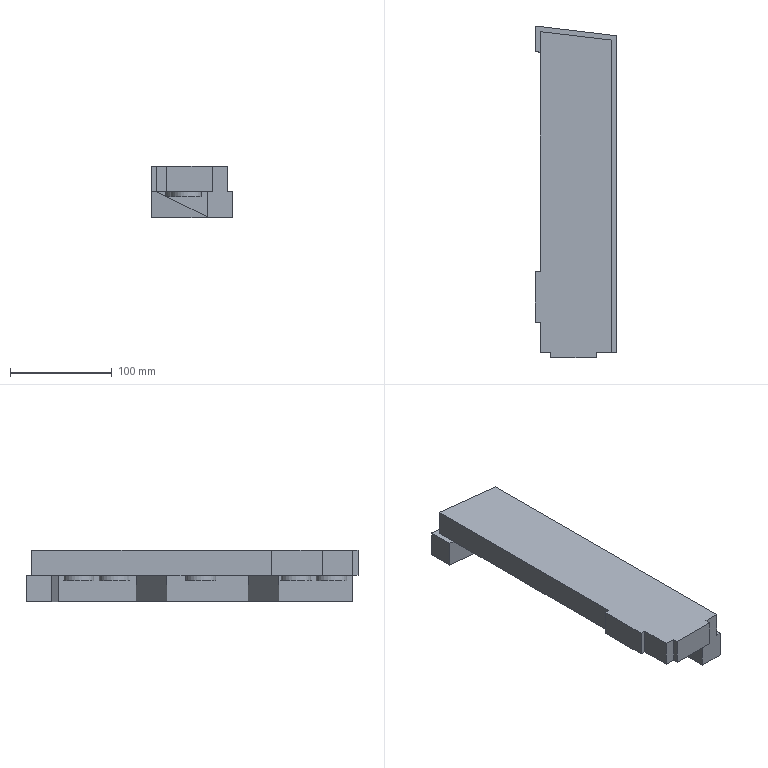Part | NX | features solid 2 | 1 solid | 39 faces | box 80 x 326.236 x 51 mm | volume 852017 mm3 | plane 31 | cylinder 5 | spline 3 | commonest cylinder face diameters 30 x5
STEP:
#1=CARTESIAN_POINT('',(-400.,-457.246,20.));
#2=VERTEX_POINT('',#1);
#3=CARTESIAN_POINT('',(-400.,-480.,20.));
#4=VERTEX_POINT('',#3);
#5=CARTESIAN_POINT('',(-400.,-457.246,20.));
#6=DIRECTION('',(0.,-1.,0.));
#7=VECTOR('',#6,1000.);
#8=LINE('',#5,#7);
#9=EDGE_CURVE('',#2,#4,#8,.T.);
#10=ORIENTED_EDGE('',*,*,#9,.T.);
#11=CARTESIAN_POINT('',(-400.,-480.,45.));
#12=VERTEX_POINT('',#11);
#13=CARTESIAN_POINT('',(-400.,-480.,20.));
#14=DIRECTION('',(0.,0.,-1.));
#15=VECTOR('',#14,1000.);
#16=LINE('',#13,#15);
#17=EDGE_CURVE('',#4,#12,#16,.F.);
#18=ORIENTED_EDGE('',*,*,#17,.T.);
#19=CARTESIAN_POINT('',(-400.,-244.365,45.));
#20=VERTEX_POINT('',#19);
#21=CARTESIAN_POINT('',(-400.,-330.218,45.));
#22=DIRECTION('',(0.,1.,0.));
#23=VECTOR('',#22,1000.);
#24=LINE('',#21,#23);
#25=EDGE_CURVE('',#12,#20,#24,.T.);
#26=ORIENTED_EDGE('',*,*,#25,.T.);
#27=CARTESIAN_POINT('',(-400.,-244.365,20.));
#28=VERTEX_POINT('',#27);
#29=CARTESIAN_POINT('',(-400.,-244.365,32.5));
#30=DIRECTION('',(0.,0.,-1.));
#31=VECTOR('',#30,1000.);
#32=LINE('',#29,#31);
#33=EDGE_CURVE('',#20,#28,#32,.T.);
#34=ORIENTED_EDGE('',*,*,#33,.T.);
#35=CARTESIAN_POINT('',(-400.,-264.493,20.));
#36=VERTEX_POINT('',#35);
#37=CARTESIAN_POINT('',(-400.,-330.218,20.));
#38=DIRECTION('',(0.,1.,0.));
#39=VECTOR('',#38,1000.);
#40=LINE('',#37,#39);
#41=EDGE_CURVE('',#36,#28,#40,.T.);
#42=ORIENTED_EDGE('',*,*,#41,.F.);
#43=CARTESIAN_POINT('',(-400.,-347.246,20.));
#44=VERTEX_POINT('',#43);
#45=CARTESIAN_POINT('',(-400.,-330.218,20.));
#46=DIRECTION('',(0.,1.,0.));
#47=VECTOR('',#46,1000.);
#48=LINE('',#45,#47);
#49=EDGE_CURVE('',#44,#36,#48,.T.);
#50=ORIENTED_EDGE('',*,*,#49,.F.);
#51=CARTESIAN_POINT('',(-400.,-377.246,20.));
#52=VERTEX_POINT('',#51);
#53=CARTESIAN_POINT('',(-400.,-347.246,20.));
#54=DIRECTION('',(0.,-1.,0.));
#55=VECTOR('',#54,1000.);
#56=LINE('',#53,#55);
#57=EDGE_CURVE('',#44,#52,#56,.T.);
#58=ORIENTED_EDGE('',*,*,#57,.T.);
#59=CARTESIAN_POINT('',(-400.,-330.218,20.));
#60=DIRECTION('',(0.,1.,0.));
#61=VECTOR('',#60,1000.);
#62=LINE('',#59,#61);
#63=EDGE_CURVE('',#2,#52,#62,.T.);
#64=ORIENTED_EDGE('',*,*,#63,.F.);
#65=EDGE_LOOP('',(#10,#18,#26,#34,#42,#50,#58,#64));
#66=FACE_BOUND('',#65,.T.);
#67=CARTESIAN_POINT('',(-400.,-330.218,45.));
#68=DIRECTION('',(-1.,0.,0.));
#69=DIRECTION('',(0.,0.,1.));
#70=AXIS2_PLACEMENT_3D('',#67,#68,#69);
#71=PLANE('',#70);
#72=ADVANCED_FACE('',(#66),#71,.T.);
#73=CARTESIAN_POINT('',(-390.,-560.,20.));
#74=VERTEX_POINT('',#73);
#75=CARTESIAN_POINT('',(-400.,-560.,20.));
#76=VERTEX_POINT('',#75);
#77=CARTESIAN_POINT('',(-53.05,-560.,20.));
#78=DIRECTION('',(-1.,0.,0.));
#79=VECTOR('',#78,1000.);
#80=LINE('',#77,#79);
#81=EDGE_CURVE('',#74,#76,#80,.T.);
#82=ORIENTED_EDGE('',*,*,#81,.F.);
#83=CARTESIAN_POINT('',(-390.,-560.,45.));
#84=VERTEX_POINT('',#83);
#85=CARTESIAN_POINT('',(-390.,-560.,25.));
#86=DIRECTION('',(0.,0.,-1.));
#87=VECTOR('',#86,1000.);
#88=LINE('',#85,#87);
#89=EDGE_CURVE('',#74,#84,#88,.F.);
#90=ORIENTED_EDGE('',*,*,#89,.T.);
#91=CARTESIAN_POINT('',(-400.,-560.,45.));
#92=VERTEX_POINT('',#91);
#93=CARTESIAN_POINT('',(-582.311,-560.,45.));
#94=DIRECTION('',(1.,0.,0.));
#95=VECTOR('',#94,1000.);
#96=LINE('',#93,#95);
#97=EDGE_CURVE('',#84,#92,#96,.F.);
#98=ORIENTED_EDGE('',*,*,#97,.T.);
#99=CARTESIAN_POINT('',(-400.,-560.,25.));
#100=DIRECTION('',(0.,0.,-1.));
#101=VECTOR('',#100,1000.);
#102=LINE('',#99,#101);
#103=EDGE_CURVE('',#76,#92,#102,.F.);
#104=ORIENTED_EDGE('',*,*,#103,.F.);
#105=EDGE_LOOP('',(#82,#90,#98,#104));
#106=FACE_BOUND('',#105,.T.);
#107=CARTESIAN_POINT('',(-325.,-560.,25.));
#108=DIRECTION('',(0.,-1.,0.));
#109=DIRECTION('',(0.,0.,-1.));
#110=AXIS2_PLACEMENT_3D('',#107,#108,#109);
#111=PLANE('',#110);
#112=ADVANCED_FACE('',(#106),#111,.T.);
#113=CARTESIAN_POINT('',(-350.,-270.257,20.));
#114=VERTEX_POINT('',#113);
#115=CARTESIAN_POINT('',(-350.,-347.246,20.));
#116=VERTEX_POINT('',#115);
#117=CARTESIAN_POINT('',(-350.,-401.561,20.));
#118=DIRECTION('',(0.,1.,0.));
#119=VECTOR('',#118,1000.);
#120=LINE('',#117,#119);
#121=EDGE_CURVE('',#114,#116,#120,.F.);
#122=ORIENTED_EDGE('',*,*,#121,.T.);
#123=CARTESIAN_POINT('',(-350.,-347.246,20.));
#124=DIRECTION('',(-1.,0.,0.));
#125=VECTOR('',#124,1000.);
#126=LINE('',#123,#125);
#127=EDGE_CURVE('',#116,#44,#126,.T.);
#128=ORIENTED_EDGE('',*,*,#127,.T.);
#129=ORIENTED_EDGE('',*,*,#49,.T.);
#130=CARTESIAN_POINT('',(-350.,-270.257,20.));
#131=CARTESIAN_POINT('',(-366.651,-268.199,20.));
#132=CARTESIAN_POINT('',(-383.329,-266.375,20.));
#133=CARTESIAN_POINT('',(-400.,-264.493,20.));
#134=B_SPLINE_CURVE_WITH_KNOTS('',3,(#130,#131,#132,#133),.UNSPECIFIED.,.F.,.F.,(4,4),(1.25,1.3),.UNSPECIFIED.);
#135=EDGE_CURVE('',#114,#36,#134,.T.);
#136=ORIENTED_EDGE('',*,*,#135,.F.);
#137=EDGE_LOOP('',(#122,#128,#129,#136));
#138=FACE_BOUND('',#137,.T.);
#139=CARTESIAN_POINT('',(-390.611,-325.558,20.));
#140=VERTEX_POINT('',#139);
#141=CARTESIAN_POINT('',(-375.611,-325.558,20.));
#142=DIRECTION('',(0.,0.,-1.));
#143=DIRECTION('',(-1.,0.,0.));
#144=AXIS2_PLACEMENT_3D('',#141,#142,#143);
#145=CIRCLE('',#144,15.);
#146=EDGE_CURVE('',#140,#140,#145,.T.);
#147=ORIENTED_EDGE('',*,*,#146,.F.);
#148=EDGE_LOOP('',(#147));
#149=FACE_BOUND('',#148,.T.);
#150=CARTESIAN_POINT('',(-385.611,-290.558,20.));
#151=VERTEX_POINT('',#150);
#152=CARTESIAN_POINT('',(-370.611,-290.558,20.));
#153=DIRECTION('',(0.,0.,-1.));
#154=DIRECTION('',(-1.,0.,0.));
#155=AXIS2_PLACEMENT_3D('',#152,#153,#154);
#156=CIRCLE('',#155,15.);
#157=EDGE_CURVE('',#151,#151,#156,.T.);
#158=ORIENTED_EDGE('',*,*,#157,.F.);
#159=EDGE_LOOP('',(#158));
#160=FACE_BOUND('',#159,.T.);
#161=CARTESIAN_POINT('',(-53.05,-401.561,20.));
#162=DIRECTION('',(0.,0.,-1.));
#163=DIRECTION('',(-1.,0.,0.));
#164=AXIS2_PLACEMENT_3D('',#161,#162,#163);
#165=PLANE('',#164);
#166=ADVANCED_FACE('',(#138,#149,#160),#165,.T.);
#167=CARTESIAN_POINT('',(-390.611,-410.558,20.));
#168=VERTEX_POINT('',#167);
#169=CARTESIAN_POINT('',(-375.611,-410.558,20.));
#170=DIRECTION('',(0.,0.,-1.));
#171=DIRECTION('',(-1.,0.,0.));
#172=AXIS2_PLACEMENT_3D('',#169,#170,#171);
#173=CIRCLE('',#172,15.);
#174=EDGE_CURVE('',#168,#168,#173,.T.);
#175=ORIENTED_EDGE('',*,*,#174,.F.);
#176=EDGE_LOOP('',(#175));
#177=FACE_BOUND('',#176,.T.);
#178=CARTESIAN_POINT('',(-350.,-377.246,20.));
#179=VERTEX_POINT('',#178);
#180=CARTESIAN_POINT('',(-350.,-457.246,20.));
#181=VERTEX_POINT('',#180);
#182=CARTESIAN_POINT('',(-350.,-401.561,20.));
#183=DIRECTION('',(0.,1.,0.));
#184=VECTOR('',#183,1000.);
#185=LINE('',#182,#184);
#186=EDGE_CURVE('',#179,#181,#185,.F.);
#187=ORIENTED_EDGE('',*,*,#186,.T.);
#188=CARTESIAN_POINT('',(-350.,-457.246,20.));
#189=DIRECTION('',(-1.,0.,0.));
#190=VECTOR('',#189,1000.);
#191=LINE('',#188,#190);
#192=EDGE_CURVE('',#181,#2,#191,.T.);
#193=ORIENTED_EDGE('',*,*,#192,.T.);
#194=ORIENTED_EDGE('',*,*,#63,.T.);
#195=CARTESIAN_POINT('',(-350.,-377.246,20.));
#196=DIRECTION('',(-1.,0.,0.));
#197=VECTOR('',#196,1000.);
#198=LINE('',#195,#197);
#199=EDGE_CURVE('',#179,#52,#198,.T.);
#200=ORIENTED_EDGE('',*,*,#199,.F.);
#201=EDGE_LOOP('',(#187,#193,#194,#200));
#202=FACE_BOUND('',#201,.T.);
#203=CARTESIAN_POINT('',(-53.05,-401.561,20.));
#204=DIRECTION('',(0.,0.,-1.));
#205=DIRECTION('',(-1.,0.,0.));
#206=AXIS2_PLACEMENT_3D('',#203,#204,#205);
#207=PLANE('',#206);
#208=ADVANCED_FACE('',(#177,#202),#207,.T.);
#209=CARTESIAN_POINT('',(-390.611,-503.935,20.));
#210=VERTEX_POINT('',#209);
#211=CARTESIAN_POINT('',(-375.611,-503.935,20.));
#212=DIRECTION('',(0.,0.,-1.));
#213=DIRECTION('',(-1.,0.,0.));
#214=AXIS2_PLACEMENT_3D('',#211,#212,#213);
#215=CIRCLE('',#214,15.);
#216=EDGE_CURVE('',#210,#210,#215,.T.);
#217=ORIENTED_EDGE('',*,*,#216,.F.);
#218=EDGE_LOOP('',(#217));
#219=FACE_BOUND('',#218,.T.);
#220=CARTESIAN_POINT('',(-400.,-530.,20.));
#221=VERTEX_POINT('',#220);
#222=CARTESIAN_POINT('',(-400.,-330.218,20.));
#223=DIRECTION('',(0.,1.,0.));
#224=VECTOR('',#223,1000.);
#225=LINE('',#222,#224);
#226=EDGE_CURVE('',#76,#221,#225,.T.);
#227=ORIENTED_EDGE('',*,*,#226,.T.);
#228=CARTESIAN_POINT('',(-405.,-530.,20.));
#229=VERTEX_POINT('',#228);
#230=CARTESIAN_POINT('',(-400.,-530.,20.));
#231=DIRECTION('',(-1.,0.,0.));
#232=VECTOR('',#231,1000.);
#233=LINE('',#230,#232);
#234=EDGE_CURVE('',#221,#229,#233,.T.);
#235=ORIENTED_EDGE('',*,*,#234,.T.);
#236=CARTESIAN_POINT('',(-405.,-480.,20.));
#237=VERTEX_POINT('',#236);
#238=CARTESIAN_POINT('',(-405.,-530.,20.));
#239=DIRECTION('',(0.,1.,0.));
#240=VECTOR('',#239,1000.);
#241=LINE('',#238,#240);
#242=EDGE_CURVE('',#229,#237,#241,.T.);
#243=ORIENTED_EDGE('',*,*,#242,.T.);
#244=CARTESIAN_POINT('',(-400.,-480.,20.));
#245=DIRECTION('',(1.,0.,0.));
#246=VECTOR('',#245,1000.);
#247=LINE('',#244,#246);
#248=EDGE_CURVE('',#4,#237,#247,.F.);
#249=ORIENTED_EDGE('',*,*,#248,.F.);
#250=CARTESIAN_POINT('',(-400.,-487.246,20.));
#251=VERTEX_POINT('',#250);
#252=CARTESIAN_POINT('',(-400.,-457.246,20.));
#253=DIRECTION('',(0.,-1.,0.));
#254=VECTOR('',#253,1000.);
#255=LINE('',#252,#254);
#256=EDGE_CURVE('',#4,#251,#255,.T.);
#257=ORIENTED_EDGE('',*,*,#256,.T.);
#258=CARTESIAN_POINT('',(-350.,-487.246,20.));
#259=VERTEX_POINT('',#258);
#260=CARTESIAN_POINT('',(-350.,-487.246,20.));
#261=DIRECTION('',(-1.,0.,0.));
#262=VECTOR('',#261,1000.);
#263=LINE('',#260,#262);
#264=EDGE_CURVE('',#259,#251,#263,.T.);
#265=ORIENTED_EDGE('',*,*,#264,.F.);
#266=CARTESIAN_POINT('',(-350.,-560.,20.));
#267=VERTEX_POINT('',#266);
#268=CARTESIAN_POINT('',(-350.,-401.561,20.));
#269=DIRECTION('',(0.,1.,0.));
#270=VECTOR('',#269,1000.);
#271=LINE('',#268,#270);
#272=EDGE_CURVE('',#259,#267,#271,.F.);
#273=ORIENTED_EDGE('',*,*,#272,.T.);
#274=CARTESIAN_POINT('',(-345.,-560.,20.));
#275=VERTEX_POINT('',#274);
#276=CARTESIAN_POINT('',(-53.05,-560.,20.));
#277=DIRECTION('',(-1.,0.,0.));
#278=VECTOR('',#277,1000.);
#279=LINE('',#276,#278);
#280=EDGE_CURVE('',#275,#267,#279,.T.);
#281=ORIENTED_EDGE('',*,*,#280,.F.);
#282=CARTESIAN_POINT('',(-345.,-565.,20.));
#283=VERTEX_POINT('',#282);
#284=CARTESIAN_POINT('',(-345.,-565.,20.));
#285=DIRECTION('',(0.,1.,0.));
#286=VECTOR('',#285,1000.);
#287=LINE('',#284,#286);
#288=EDGE_CURVE('',#283,#275,#287,.T.);
#289=ORIENTED_EDGE('',*,*,#288,.F.);
#290=CARTESIAN_POINT('',(-390.,-565.,20.));
#291=VERTEX_POINT('',#290);
#292=CARTESIAN_POINT('',(-53.05,-565.,20.));
#293=DIRECTION('',(-1.,0.,0.));
#294=VECTOR('',#293,1000.);
#295=LINE('',#292,#294);
#296=EDGE_CURVE('',#283,#291,#295,.T.);
#297=ORIENTED_EDGE('',*,*,#296,.T.);
#298=CARTESIAN_POINT('',(-390.,-565.,20.));
#299=DIRECTION('',(0.,1.,0.));
#300=VECTOR('',#299,1000.);
#301=LINE('',#298,#300);
#302=EDGE_CURVE('',#291,#74,#301,.T.);
#303=ORIENTED_EDGE('',*,*,#302,.T.);
#304=ORIENTED_EDGE('',*,*,#81,.T.);
#305=EDGE_LOOP('',(#227,#235,#243,#249,#257,#265,#273,#281,#289,#297,#303,#304));
#306=FACE_BOUND('',#305,.T.);
#307=CARTESIAN_POINT('',(-385.611,-538.935,20.));
#308=VERTEX_POINT('',#307);
#309=CARTESIAN_POINT('',(-370.611,-538.935,20.));
#310=DIRECTION('',(0.,0.,-1.));
#311=DIRECTION('',(-1.,0.,0.));
#312=AXIS2_PLACEMENT_3D('',#309,#310,#311);
#313=CIRCLE('',#312,15.);
#314=EDGE_CURVE('',#308,#308,#313,.T.);
#315=ORIENTED_EDGE('',*,*,#314,.F.);
#316=EDGE_LOOP('',(#315));
#317=FACE_BOUND('',#316,.T.);
#318=CARTESIAN_POINT('',(-53.05,-401.561,20.));
#319=DIRECTION('',(0.,0.,-1.));
#320=DIRECTION('',(-1.,0.,0.));
#321=AXIS2_PLACEMENT_3D('',#318,#319,#320);
#322=PLANE('',#321);
#323=ADVANCED_FACE('',(#219,#306,#317),#322,.T.);
#324=CARTESIAN_POINT('',(-330.,-560.,45.));
#325=VERTEX_POINT('',#324);
#326=CARTESIAN_POINT('',(-345.,-560.,45.));
#327=VERTEX_POINT('',#326);
#328=CARTESIAN_POINT('',(-582.311,-560.,45.));
#329=DIRECTION('',(1.,0.,0.));
#330=VECTOR('',#329,1000.);
#331=LINE('',#328,#330);
#332=EDGE_CURVE('',#325,#327,#331,.F.);
#333=ORIENTED_EDGE('',*,*,#332,.T.);
#334=CARTESIAN_POINT('',(-345.,-560.,25.));
#335=DIRECTION('',(0.,0.,1.));
#336=VECTOR('',#335,1000.);
#337=LINE('',#334,#336);
#338=EDGE_CURVE('',#327,#275,#337,.F.);
#339=ORIENTED_EDGE('',*,*,#338,.T.);
#340=ORIENTED_EDGE('',*,*,#280,.T.);
#341=CARTESIAN_POINT('',(-350.,-560.,-6.));
#342=VERTEX_POINT('',#341);
#343=CARTESIAN_POINT('',(-350.,-560.,25.));
#344=DIRECTION('',(0.,0.,-1.));
#345=VECTOR('',#344,1000.);
#346=LINE('',#343,#345);
#347=EDGE_CURVE('',#267,#342,#346,.T.);
#348=ORIENTED_EDGE('',*,*,#347,.T.);
#349=CARTESIAN_POINT('',(-325.,-560.,-6.));
#350=VERTEX_POINT('',#349);
#351=CARTESIAN_POINT('',(-582.311,-560.,-6.));
#352=DIRECTION('',(1.,0.,0.));
#353=VECTOR('',#352,1000.);
#354=LINE('',#351,#353);
#355=EDGE_CURVE('',#350,#342,#354,.F.);
#356=ORIENTED_EDGE('',*,*,#355,.F.);
#357=CARTESIAN_POINT('',(-325.,-560.,20.));
#358=VERTEX_POINT('',#357);
#359=CARTESIAN_POINT('',(-325.,-560.,25.));
#360=DIRECTION('',(0.,0.,1.));
#361=VECTOR('',#360,1000.);
#362=LINE('',#359,#361);
#363=EDGE_CURVE('',#358,#350,#362,.F.);
#364=ORIENTED_EDGE('',*,*,#363,.F.);
#365=CARTESIAN_POINT('',(-330.,-560.,20.));
#366=VERTEX_POINT('',#365);
#367=CARTESIAN_POINT('',(-325.,-560.,20.));
#368=DIRECTION('',(-1.,0.,0.));
#369=VECTOR('',#368,1000.);
#370=LINE('',#367,#369);
#371=EDGE_CURVE('',#358,#366,#370,.T.);
#372=ORIENTED_EDGE('',*,*,#371,.T.);
#373=CARTESIAN_POINT('',(-330.,-560.,25.));
#374=DIRECTION('',(0.,0.,-1.));
#375=VECTOR('',#374,1000.);
#376=LINE('',#373,#375);
#377=EDGE_CURVE('',#325,#366,#376,.T.);
#378=ORIENTED_EDGE('',*,*,#377,.F.);
#379=EDGE_LOOP('',(#333,#339,#340,#348,#356,#364,#372,#378));
#380=FACE_BOUND('',#379,.T.);
#381=CARTESIAN_POINT('',(-325.,-560.,25.));
#382=DIRECTION('',(0.,-1.,0.));
#383=DIRECTION('',(0.,0.,-1.));
#384=AXIS2_PLACEMENT_3D('',#381,#382,#383);
#385=PLANE('',#384);
#386=ADVANCED_FACE('',(#380),#385,.T.);
#387=ORIENTED_EDGE('',*,*,#33,.F.);
#388=CARTESIAN_POINT('',(-330.,-252.678,45.));
#389=VERTEX_POINT('',#388);
#390=CARTESIAN_POINT('',(-330.,-252.678,45.));
#391=CARTESIAN_POINT('',(-332.478,-252.342,45.));
#392=CARTESIAN_POINT('',(-337.652,-251.655,45.));
#393=CARTESIAN_POINT('',(-344.665,-250.765,45.));
#394=CARTESIAN_POINT('',(-350.603,-250.033,45.));
#395=CARTESIAN_POINT('',(-354.452,-249.568,45.));
#396=CARTESIAN_POINT('',(-357.611,-249.191,45.));
#397=CARTESIAN_POINT('',(-360.025,-248.906,45.));
#398=CARTESIAN_POINT('',(-362.061,-248.667,45.));
#399=CARTESIAN_POINT('',(-363.523,-248.497,45.));
#400=CARTESIAN_POINT('',(-364.333,-248.402,45.));
#401=CARTESIAN_POINT('',(-365.03,-248.322,45.));
#402=CARTESIAN_POINT('',(-365.396,-248.279,45.));
#403=CARTESIAN_POINT('',(-366.012,-248.208,45.));
#404=CARTESIAN_POINT('',(-367.059,-248.087,45.));
#405=CARTESIAN_POINT('',(-368.655,-247.904,45.));
#406=CARTESIAN_POINT('',(-370.671,-247.673,45.));
#407=CARTESIAN_POINT('',(-372.804,-247.43,45.));
#408=CARTESIAN_POINT('',(-375.049,-247.175,45.));
#409=CARTESIAN_POINT('',(-377.015,-246.952,45.));
#410=CARTESIAN_POINT('',(-378.645,-246.768,45.));
#411=CARTESIAN_POINT('',(-379.894,-246.627,45.));
#412=CARTESIAN_POINT('',(-380.967,-246.506,45.));
#413=CARTESIAN_POINT('',(-381.712,-246.423,45.));
#414=CARTESIAN_POINT('',(-382.17,-246.371,45.));
#415=CARTESIAN_POINT('',(-382.435,-246.341,45.));
#416=CARTESIAN_POINT('',(-383.006,-246.277,45.));
#417=CARTESIAN_POINT('',(-383.648,-246.205,45.));
#418=CARTESIAN_POINT('',(-384.797,-246.076,45.));
#419=CARTESIAN_POINT('',(-386.338,-245.902,45.));
#420=CARTESIAN_POINT('',(-388.081,-245.706,45.));
#421=CARTESIAN_POINT('',(-390.244,-245.463,45.));
#422=CARTESIAN_POINT('',(-392.656,-245.192,45.));
#423=CARTESIAN_POINT('',(-395.888,-244.828,45.));
#424=CARTESIAN_POINT('',(-398.754,-244.506,45.));
#425=CARTESIAN_POINT('',(-399.793,-244.389,45.));
#426=CARTESIAN_POINT('',(-400.,-244.365,45.));
#427=B_SPLINE_CURVE_WITH_KNOTS('',3,(#390,#391,#392,#393,#394,#395,#396,#397,#398,#399,#400,#401,#402,#403,#404,#405,#406,#407,#408,#409,#410,#411,#412,#413,#414,#415,#416,#417,#418,#419,#420,#421,#422,#423,#424,#425,#426),.UNSPECIFIED.,.F.,.F.,(4,1,1,1,1,1,1,1,1,1,1,1,1,1,1,1,1,1,1,1,1,1,1,1,1,1,1,1,1,1,1,1,1,1,4),(0.,0.125,0.25,0.3125,0.375,0.4062,0.4375,0.4688,0.4844,0.4922,0.5,0.5078,0.5156,0.5312,0.5625,0.5938,0.625,0.6562,0.6875,0.7031,0.7188,0.7344,0.7422,0.7461,0.75,0.7539,0.7578,0.7656,0.7812,0.7969,0.8125,0.8438,0.875,0.9375,1.),.UNSPECIFIED.);
#428=EDGE_CURVE('',#389,#20,#427,.T.);
#429=ORIENTED_EDGE('',*,*,#428,.F.);
#430=CARTESIAN_POINT('',(-330.,-252.678,20.));
#431=VERTEX_POINT('',#430);
#432=CARTESIAN_POINT('',(-330.,-252.678,32.5));
#433=DIRECTION('',(0.,0.,-1.));
#434=VECTOR('',#433,1000.);
#435=LINE('',#432,#434);
#436=EDGE_CURVE('',#389,#431,#435,.T.);
#437=ORIENTED_EDGE('',*,*,#436,.T.);
#438=CARTESIAN_POINT('',(-330.,-252.678,20.));
#439=CARTESIAN_POINT('',(-353.282,-249.514,20.));
#440=CARTESIAN_POINT('',(-376.65,-247.01,20.));
#441=CARTESIAN_POINT('',(-400.,-244.365,20.));
#442=B_SPLINE_CURVE_WITH_KNOTS('',3,(#438,#439,#440,#441),.UNSPECIFIED.,.F.,.F.,(4,4),(1.234,1.304),.UNSPECIFIED.);
#443=EDGE_CURVE('',#431,#28,#442,.T.);
#444=ORIENTED_EDGE('',*,*,#443,.T.);
#445=EDGE_LOOP('',(#387,#429,#437,#444));
#446=FACE_BOUND('',#445,.T.);
#447=CARTESIAN_POINT('',(-330.,-252.678,45.));
#448=CARTESIAN_POINT('',(-330.,-252.678,20.));
#449=CARTESIAN_POINT('',(-353.225,-249.521,45.));
#450=CARTESIAN_POINT('',(-353.225,-249.521,20.));
#451=CARTESIAN_POINT('',(-376.596,-247.016,45.));
#452=CARTESIAN_POINT('',(-376.596,-247.016,20.));
#453=CARTESIAN_POINT('',(-400.,-244.365,45.));
#454=CARTESIAN_POINT('',(-400.,-244.365,20.));
#455=B_SPLINE_SURFACE_WITH_KNOTS('',3,1,((#447,#448),(#449,#450),(#451,#452),(#453,#454)),.SURF_OF_LINEAR_EXTRUSION.,.F.,.F.,.F.,(4,4),(2,2),(0.185,0.4245),(0.,1.),.PIECEWISE_BEZIER_KNOTS.);
#456=ADVANCED_FACE('',(#446),#455,.F.);
#457=ORIENTED_EDGE('',*,*,#428,.T.);
#458=ORIENTED_EDGE('',*,*,#25,.F.);
#459=CARTESIAN_POINT('',(-405.,-480.,45.));
#460=VERTEX_POINT('',#459);
#461=CARTESIAN_POINT('',(-400.,-480.,45.));
#462=DIRECTION('',(1.,0.,0.));
#463=VECTOR('',#462,1000.);
#464=LINE('',#461,#463);
#465=EDGE_CURVE('',#12,#460,#464,.F.);
#466=ORIENTED_EDGE('',*,*,#465,.T.);
#467=CARTESIAN_POINT('',(-405.,-530.,45.));
#468=VERTEX_POINT('',#467);
#469=CARTESIAN_POINT('',(-405.,-530.,45.));
#470=DIRECTION('',(0.,1.,0.));
#471=VECTOR('',#470,1000.);
#472=LINE('',#469,#471);
#473=EDGE_CURVE('',#468,#460,#472,.T.);
#474=ORIENTED_EDGE('',*,*,#473,.F.);
#475=CARTESIAN_POINT('',(-400.,-530.,45.));
#476=VERTEX_POINT('',#475);
#477=CARTESIAN_POINT('',(-400.,-530.,45.));
#478=DIRECTION('',(-1.,0.,0.));
#479=VECTOR('',#478,1000.);
#480=LINE('',#477,#479);
#481=EDGE_CURVE('',#476,#468,#480,.T.);
#482=ORIENTED_EDGE('',*,*,#481,.F.);
#483=CARTESIAN_POINT('',(-400.,-330.218,45.));
#484=DIRECTION('',(0.,1.,0.));
#485=VECTOR('',#484,1000.);
#486=LINE('',#483,#485);
#487=EDGE_CURVE('',#92,#476,#486,.T.);
#488=ORIENTED_EDGE('',*,*,#487,.F.);
#489=ORIENTED_EDGE('',*,*,#97,.F.);
#490=CARTESIAN_POINT('',(-390.,-565.,45.));
#491=VERTEX_POINT('',#490);
#492=CARTESIAN_POINT('',(-390.,-565.,45.));
#493=DIRECTION('',(0.,1.,0.));
#494=VECTOR('',#493,1000.);
#495=LINE('',#492,#494);
#496=EDGE_CURVE('',#491,#84,#495,.T.);
#497=ORIENTED_EDGE('',*,*,#496,.F.);
#498=CARTESIAN_POINT('',(-345.,-565.,45.));
#499=VERTEX_POINT('',#498);
#500=CARTESIAN_POINT('',(-582.311,-565.,45.));
#501=DIRECTION('',(1.,0.,0.));
#502=VECTOR('',#501,1000.);
#503=LINE('',#500,#502);
#504=EDGE_CURVE('',#499,#491,#503,.F.);
#505=ORIENTED_EDGE('',*,*,#504,.F.);
#506=CARTESIAN_POINT('',(-345.,-565.,45.));
#507=DIRECTION('',(0.,1.,0.));
#508=VECTOR('',#507,1000.);
#509=LINE('',#506,#508);
#510=EDGE_CURVE('',#499,#327,#509,.T.);
#511=ORIENTED_EDGE('',*,*,#510,.T.);
#512=ORIENTED_EDGE('',*,*,#332,.F.);
#513=CARTESIAN_POINT('',(-330.,-348.688,45.));
#514=DIRECTION('',(0.,1.,0.));
#515=VECTOR('',#514,1000.);
#516=LINE('',#513,#515);
#517=EDGE_CURVE('',#325,#389,#516,.T.);
#518=ORIENTED_EDGE('',*,*,#517,.T.);
#519=EDGE_LOOP('',(#457,#458,#466,#474,#482,#488,#489,#497,#505,#511,#512,#518));
#520=FACE_BOUND('',#519,.T.);
#521=CARTESIAN_POINT('',(-582.311,-1052.635,45.));
#522=DIRECTION('',(0.,0.,1.));
#523=DIRECTION('',(1.,0.,0.));
#524=AXIS2_PLACEMENT_3D('',#521,#522,#523);
#525=PLANE('',#524);
#526=ADVANCED_FACE('',(#520),#525,.T.);
#527=CARTESIAN_POINT('',(-325.,-248.32,20.));
#528=VERTEX_POINT('',#527);
#529=CARTESIAN_POINT('',(-325.,-401.561,20.));
#530=DIRECTION('',(0.,1.,0.));
#531=VECTOR('',#530,1000.);
#532=LINE('',#529,#531);
#533=EDGE_CURVE('',#528,#358,#532,.F.);
#534=ORIENTED_EDGE('',*,*,#533,.T.);
#535=ORIENTED_EDGE('',*,*,#363,.T.);
#536=CARTESIAN_POINT('',(-325.,-248.32,-6.));
#537=VERTEX_POINT('',#536);
#538=CARTESIAN_POINT('',(-325.,-1052.635,-6.));
#539=DIRECTION('',(0.,1.,0.));
#540=VECTOR('',#539,1000.);
#541=LINE('',#538,#540);
#542=EDGE_CURVE('',#350,#537,#541,.T.);
#543=ORIENTED_EDGE('',*,*,#542,.T.);
#544=CARTESIAN_POINT('',(-325.,-248.32,7.));
#545=DIRECTION('',(0.,0.,-1.));
#546=VECTOR('',#545,1000.);
#547=LINE('',#544,#546);
#548=EDGE_CURVE('',#537,#528,#547,.F.);
#549=ORIENTED_EDGE('',*,*,#548,.T.);
#550=EDGE_LOOP('',(#534,#535,#543,#549));
#551=FACE_BOUND('',#550,.T.);
#552=CARTESIAN_POINT('',(-325.,-560.,0.));
#553=DIRECTION('',(1.,0.,0.));
#554=DIRECTION('',(0.,0.,-1.));
#555=AXIS2_PLACEMENT_3D('',#552,#553,#554);
#556=PLANE('',#555);
#557=ADVANCED_FACE('',(#551),#556,.T.);
#558=ORIENTED_EDGE('',*,*,#377,.T.);
#559=CARTESIAN_POINT('',(-330.,-348.688,20.));
#560=DIRECTION('',(0.,1.,0.));
#561=VECTOR('',#560,1000.);
#562=LINE('',#559,#561);
#563=EDGE_CURVE('',#366,#431,#562,.T.);
#564=ORIENTED_EDGE('',*,*,#563,.T.);
#565=ORIENTED_EDGE('',*,*,#436,.F.);
#566=ORIENTED_EDGE('',*,*,#517,.F.);
#567=EDGE_LOOP('',(#558,#564,#565,#566));
#568=FACE_BOUND('',#567,.T.);
#569=CARTESIAN_POINT('',(-330.,-348.688,45.));
#570=DIRECTION('',(-1.,0.,0.));
#571=DIRECTION('',(0.,0.,1.));
#572=AXIS2_PLACEMENT_3D('',#569,#570,#571);
#573=PLANE('',#572);
#574=ADVANCED_FACE('',(#568),#573,.F.);
#575=CARTESIAN_POINT('',(-350.,-457.246,-5.));
#576=VERTEX_POINT('',#575);
#577=CARTESIAN_POINT('',(-350.,-457.246,20.));
#578=DIRECTION('',(0.,0.,-1.));
#579=VECTOR('',#578,1000.);
#580=LINE('',#577,#579);
#581=EDGE_CURVE('',#181,#576,#580,.T.);
#582=ORIENTED_EDGE('',*,*,#581,.F.);
#583=ORIENTED_EDGE('',*,*,#186,.F.);
#584=CARTESIAN_POINT('',(-350.,-377.246,-5.));
#585=VERTEX_POINT('',#584);
#586=CARTESIAN_POINT('',(-350.,-377.246,20.));
#587=DIRECTION('',(0.,0.,-1.));
#588=VECTOR('',#587,1000.);
#589=LINE('',#586,#588);
#590=EDGE_CURVE('',#179,#585,#589,.T.);
#591=ORIENTED_EDGE('',*,*,#590,.T.);
#592=CARTESIAN_POINT('',(-350.,-347.246,-5.));
#593=VERTEX_POINT('',#592);
#594=CARTESIAN_POINT('',(-350.,-347.246,-5.));
#595=DIRECTION('',(0.,1.,0.));
#596=VECTOR('',#595,1000.);
#597=LINE('',#594,#596);
#598=EDGE_CURVE('',#593,#585,#597,.F.);
#599=ORIENTED_EDGE('',*,*,#598,.F.);
#600=CARTESIAN_POINT('',(-350.,-347.246,20.));
#601=DIRECTION('',(0.,0.,-1.));
#602=VECTOR('',#601,1000.);
#603=LINE('',#600,#602);
#604=EDGE_CURVE('',#116,#593,#603,.T.);
#605=ORIENTED_EDGE('',*,*,#604,.F.);
#606=ORIENTED_EDGE('',*,*,#121,.F.);
#607=CARTESIAN_POINT('',(-350.,-270.257,-6.));
#608=VERTEX_POINT('',#607);
#609=CARTESIAN_POINT('',(-350.,-270.257,7.));
#610=DIRECTION('',(0.,0.,1.));
#611=VECTOR('',#610,1000.);
#612=LINE('',#609,#611);
#613=EDGE_CURVE('',#608,#114,#612,.T.);
#614=ORIENTED_EDGE('',*,*,#613,.F.);
#615=CARTESIAN_POINT('',(-350.,-1052.635,-6.));
#616=DIRECTION('',(0.,-1.,0.));
#617=VECTOR('',#616,1000.);
#618=LINE('',#615,#617);
#619=EDGE_CURVE('',#342,#608,#618,.F.);
#620=ORIENTED_EDGE('',*,*,#619,.F.);
#621=ORIENTED_EDGE('',*,*,#347,.F.);
#622=ORIENTED_EDGE('',*,*,#272,.F.);
#623=CARTESIAN_POINT('',(-350.,-487.246,-5.));
#624=VERTEX_POINT('',#623);
#625=CARTESIAN_POINT('',(-350.,-487.246,20.));
#626=DIRECTION('',(0.,0.,-1.));
#627=VECTOR('',#626,1000.);
#628=LINE('',#625,#627);
#629=EDGE_CURVE('',#259,#624,#628,.T.);
#630=ORIENTED_EDGE('',*,*,#629,.T.);
#631=CARTESIAN_POINT('',(-350.,-457.246,-5.));
#632=DIRECTION('',(0.,1.,0.));
#633=VECTOR('',#632,1000.);
#634=LINE('',#631,#633);
#635=EDGE_CURVE('',#576,#624,#634,.F.);
#636=ORIENTED_EDGE('',*,*,#635,.F.);
#637=EDGE_LOOP('',(#582,#583,#591,#599,#605,#606,#614,#620,#621,#622,#630,#636));
#638=FACE_BOUND('',#637,.T.);
#639=CARTESIAN_POINT('',(-350.,-560.,25.));
#640=DIRECTION('',(-1.,0.,0.));
#641=DIRECTION('',(0.,0.,1.));
#642=AXIS2_PLACEMENT_3D('',#639,#640,#641);
#643=PLANE('',#642);
#644=ADVANCED_FACE('',(#638),#643,.T.);
#645=CARTESIAN_POINT('',(-405.,-238.764,20.));
#646=VERTEX_POINT('',#645);
#647=CARTESIAN_POINT('',(-405.,-263.926,20.));
#648=VERTEX_POINT('',#647);
#649=CARTESIAN_POINT('',(-405.,-401.561,20.));
#650=DIRECTION('',(0.,1.,0.));
#651=VECTOR('',#650,1000.);
#652=LINE('',#649,#651);
#653=EDGE_CURVE('',#646,#648,#652,.F.);
#654=ORIENTED_EDGE('',*,*,#653,.T.);
#655=CARTESIAN_POINT('',(-400.,-264.493,20.));
#656=CARTESIAN_POINT('',(-401.665,-264.305,20.));
#657=CARTESIAN_POINT('',(-403.332,-264.116,20.));
#658=CARTESIAN_POINT('',(-405.,-263.926,20.));
#659=B_SPLINE_CURVE_WITH_KNOTS('',3,(#655,#656,#657,#658),.UNSPECIFIED.,.F.,.F.,(4,4),(0.4169,0.4339),.UNSPECIFIED.);
#660=EDGE_CURVE('',#36,#648,#659,.T.);
#661=ORIENTED_EDGE('',*,*,#660,.F.);
#662=ORIENTED_EDGE('',*,*,#41,.T.);
#663=ORIENTED_EDGE('',*,*,#443,.F.);
#664=ORIENTED_EDGE('',*,*,#563,.F.);
#665=ORIENTED_EDGE('',*,*,#371,.F.);
#666=ORIENTED_EDGE('',*,*,#533,.F.);
#667=CARTESIAN_POINT('',(-325.,-248.32,20.));
#668=CARTESIAN_POINT('',(-351.587,-244.607,20.));
#669=CARTESIAN_POINT('',(-378.313,-241.817,20.));
#670=CARTESIAN_POINT('',(-405.,-238.764,20.));
#671=B_SPLINE_CURVE_WITH_KNOTS('',3,(#667,#668,#669,#670),.UNSPECIFIED.,.F.,.F.,(4,4),(1.144,1.22),.UNSPECIFIED.);
#672=EDGE_CURVE('',#528,#646,#671,.T.);
#673=ORIENTED_EDGE('',*,*,#672,.T.);
#674=EDGE_LOOP('',(#654,#661,#662,#663,#664,#665,#666,#673));
#675=FACE_BOUND('',#674,.T.);
#676=CARTESIAN_POINT('',(-53.05,-401.561,20.));
#677=DIRECTION('',(0.,0.,1.));
#678=DIRECTION('',(1.,0.,0.));
#679=AXIS2_PLACEMENT_3D('',#676,#677,#678);
#680=PLANE('',#679);
#681=ADVANCED_FACE('',(#675),#680,.T.);
#682=CARTESIAN_POINT('',(-405.,-238.764,-6.));
#683=VERTEX_POINT('',#682);
#684=CARTESIAN_POINT('',(-325.,-248.32,-6.));
#685=CARTESIAN_POINT('',(-351.591,-244.606,-6.));
#686=CARTESIAN_POINT('',(-378.314,-241.817,-6.));
#687=CARTESIAN_POINT('',(-405.,-238.764,-6.));
#688=B_SPLINE_CURVE_WITH_KNOTS('',3,(#684,#685,#686,#687),.UNSPECIFIED.,.F.,.F.,(4,4),(0.4868,0.5642),.UNSPECIFIED.);
#689=EDGE_CURVE('',#537,#683,#688,.T.);
#690=ORIENTED_EDGE('',*,*,#689,.T.);
#691=CARTESIAN_POINT('',(-405.,-238.764,7.));
#692=DIRECTION('',(0.,0.,-1.));
#693=VECTOR('',#692,1000.);
#694=LINE('',#691,#693);
#695=EDGE_CURVE('',#683,#646,#694,.F.);
#696=ORIENTED_EDGE('',*,*,#695,.T.);
#697=ORIENTED_EDGE('',*,*,#672,.F.);
#698=ORIENTED_EDGE('',*,*,#548,.F.);
#699=EDGE_LOOP('',(#690,#696,#697,#698));
#700=FACE_BOUND('',#699,.T.);
#701=CARTESIAN_POINT('',(-325.,-248.32,20.));
#702=CARTESIAN_POINT('',(-325.,-248.32,-6.));
#703=CARTESIAN_POINT('',(-351.598,-244.605,20.));
#704=CARTESIAN_POINT('',(-351.598,-244.605,-6.));
#705=CARTESIAN_POINT('',(-378.318,-241.817,20.));
#706=CARTESIAN_POINT('',(-378.318,-241.817,-6.));
#707=CARTESIAN_POINT('',(-405.,-238.764,20.));
#708=CARTESIAN_POINT('',(-405.,-238.764,-6.));
#709=B_SPLINE_SURFACE_WITH_KNOTS('',3,1,((#701,#702),(#703,#704),(#705,#706),(#707,#708)),.SURF_OF_LINEAR_EXTRUSION.,.F.,.F.,.F.,(4,4),(2,2),(0.5297,0.5985),(0.,1.),.PIECEWISE_BEZIER_KNOTS.);
#710=ADVANCED_FACE('',(#700),#709,.F.);
#711=ORIENTED_EDGE('',*,*,#135,.T.);
#712=ORIENTED_EDGE('',*,*,#660,.T.);
#713=CARTESIAN_POINT('',(-405.,-263.926,-6.));
#714=VERTEX_POINT('',#713);
#715=CARTESIAN_POINT('',(-405.,-263.926,7.));
#716=DIRECTION('',(0.,0.,1.));
#717=VECTOR('',#716,1000.);
#718=LINE('',#715,#717);
#719=EDGE_CURVE('',#648,#714,#718,.F.);
#720=ORIENTED_EDGE('',*,*,#719,.T.);
#721=CARTESIAN_POINT('',(-350.,-270.257,-6.));
#722=CARTESIAN_POINT('',(-368.313,-267.994,-6.));
#723=CARTESIAN_POINT('',(-386.664,-266.012,-6.));
#724=CARTESIAN_POINT('',(-405.,-263.926,-6.));
#725=B_SPLINE_CURVE_WITH_KNOTS('',3,(#721,#722,#723,#724),.UNSPECIFIED.,.F.,.F.,(4,4),(0.0701,0.1254),.UNSPECIFIED.);
#726=EDGE_CURVE('',#608,#714,#725,.T.);
#727=ORIENTED_EDGE('',*,*,#726,.F.);
#728=ORIENTED_EDGE('',*,*,#613,.T.);
#729=EDGE_LOOP('',(#711,#712,#720,#727,#728));
#730=FACE_BOUND('',#729,.T.);
#731=CARTESIAN_POINT('',(-350.,-270.257,-6.));
#732=CARTESIAN_POINT('',(-350.,-270.257,20.));
#733=CARTESIAN_POINT('',(-368.139,-268.015,-6.));
#734=CARTESIAN_POINT('',(-368.139,-268.015,20.));
#735=CARTESIAN_POINT('',(-386.491,-266.032,-6.));
#736=CARTESIAN_POINT('',(-386.491,-266.032,20.));
#737=CARTESIAN_POINT('',(-405.,-263.926,-6.));
#738=CARTESIAN_POINT('',(-405.,-263.926,20.));
#739=B_SPLINE_SURFACE_WITH_KNOTS('',3,1,((#731,#732),(#733,#734),(#735,#736),(#737,#738)),.SURF_OF_LINEAR_EXTRUSION.,.F.,.F.,.F.,(4,4),(2,2),(0.2452,0.4339),(0.,1.),.PIECEWISE_BEZIER_KNOTS.);
#740=ADVANCED_FACE('',(#730),#739,.F.);
#741=ORIENTED_EDGE('',*,*,#726,.T.);
#742=CARTESIAN_POINT('',(-405.,-1052.635,-6.));
#743=DIRECTION('',(0.,1.,0.));
#744=VECTOR('',#743,1000.);
#745=LINE('',#742,#744);
#746=EDGE_CURVE('',#714,#683,#745,.T.);
#747=ORIENTED_EDGE('',*,*,#746,.T.);
#748=ORIENTED_EDGE('',*,*,#689,.F.);
#749=ORIENTED_EDGE('',*,*,#542,.F.);
#750=ORIENTED_EDGE('',*,*,#355,.T.);
#751=ORIENTED_EDGE('',*,*,#619,.T.);
#752=EDGE_LOOP('',(#741,#747,#748,#749,#750,#751));
#753=FACE_BOUND('',#752,.T.);
#754=CARTESIAN_POINT('',(-582.311,-1052.635,-6.));
#755=DIRECTION('',(0.,0.,1.));
#756=DIRECTION('',(1.,0.,0.));
#757=AXIS2_PLACEMENT_3D('',#754,#755,#756);
#758=PLANE('',#757);
#759=ADVANCED_FACE('',(#753),#758,.F.);
#760=ORIENTED_EDGE('',*,*,#719,.F.);
#761=ORIENTED_EDGE('',*,*,#653,.F.);
#762=ORIENTED_EDGE('',*,*,#695,.F.);
#763=ORIENTED_EDGE('',*,*,#746,.F.);
#764=EDGE_LOOP('',(#760,#761,#762,#763));
#765=FACE_BOUND('',#764,.T.);
#766=CARTESIAN_POINT('',(-405.,-560.,0.));
#767=DIRECTION('',(1.,0.,0.));
#768=DIRECTION('',(0.,0.,-1.));
#769=AXIS2_PLACEMENT_3D('',#766,#767,#768);
#770=PLANE('',#769);
#771=ADVANCED_FACE('',(#765),#770,.F.);
#772=CARTESIAN_POINT('',(-400.,-530.,20.));
#773=DIRECTION('',(0.,0.,1.));
#774=VECTOR('',#773,1000.);
#775=LINE('',#772,#774);
#776=EDGE_CURVE('',#221,#476,#775,.T.);
#777=ORIENTED_EDGE('',*,*,#776,.F.);
#778=ORIENTED_EDGE('',*,*,#226,.F.);
#779=ORIENTED_EDGE('',*,*,#103,.T.);
#780=ORIENTED_EDGE('',*,*,#487,.T.);
#781=EDGE_LOOP('',(#777,#778,#779,#780));
#782=FACE_BOUND('',#781,.T.);
#783=CARTESIAN_POINT('',(-400.,-330.218,45.));
#784=DIRECTION('',(-1.,0.,0.));
#785=DIRECTION('',(0.,0.,1.));
#786=AXIS2_PLACEMENT_3D('',#783,#784,#785);
#787=PLANE('',#786);
#788=ADVANCED_FACE('',(#782),#787,.T.);
#789=CARTESIAN_POINT('',(-360.611,-325.558,15.));
#790=VERTEX_POINT('',#789);
#791=CARTESIAN_POINT('',(-375.611,-325.558,15.));
#792=DIRECTION('',(0.,0.,1.));
#793=DIRECTION('',(1.,0.,0.));
#794=AXIS2_PLACEMENT_3D('',#791,#792,#793);
#795=CIRCLE('',#794,15.);
#796=EDGE_CURVE('',#790,#790,#795,.T.);
#797=ORIENTED_EDGE('',*,*,#796,.T.);
#798=EDGE_LOOP('',(#797));
#799=FACE_BOUND('',#798,.T.);
#800=ORIENTED_EDGE('',*,*,#146,.T.);
#801=EDGE_LOOP('',(#800));
#802=FACE_BOUND('',#801,.T.);
#803=CARTESIAN_POINT('',(-375.611,-325.558,25.));
#804=DIRECTION('',(0.,0.,-1.));
#805=DIRECTION('',(-1.,0.,0.));
#806=AXIS2_PLACEMENT_3D('',#803,#804,#805);
#807=CYLINDRICAL_SURFACE('',#806,15.);
#808=ADVANCED_FACE('',(#799,#802),#807,.T.);
#809=ORIENTED_EDGE('',*,*,#796,.F.);
#810=EDGE_LOOP('',(#809));
#811=FACE_BOUND('',#810,.T.);
#812=CARTESIAN_POINT('',(-375.611,-325.558,15.));
#813=DIRECTION('',(0.,0.,1.));
#814=DIRECTION('',(1.,0.,0.));
#815=AXIS2_PLACEMENT_3D('',#812,#813,#814);
#816=PLANE('',#815);
#817=ADVANCED_FACE('',(#811),#816,.F.);
#818=ORIENTED_EDGE('',*,*,#604,.T.);
#819=CARTESIAN_POINT('',(-360.,-347.246,0.));
#820=DIRECTION('',(-0.8944,0.,0.4472));
#821=VECTOR('',#820,1000.);
#822=LINE('',#819,#821);
#823=EDGE_CURVE('',#593,#44,#822,.T.);
#824=ORIENTED_EDGE('',*,*,#823,.T.);
#825=ORIENTED_EDGE('',*,*,#127,.F.);
#826=EDGE_LOOP('',(#818,#824,#825));
#827=FACE_BOUND('',#826,.T.);
#828=CARTESIAN_POINT('',(-350.,-347.246,20.));
#829=DIRECTION('',(0.,1.,0.));
#830=DIRECTION('',(-1.,0.,0.));
#831=AXIS2_PLACEMENT_3D('',#828,#829,#830);
#832=PLANE('',#831);
#833=ADVANCED_FACE('',(#827),#832,.T.);
#834=ORIENTED_EDGE('',*,*,#199,.T.);
#835=CARTESIAN_POINT('',(-360.,-377.246,0.));
#836=DIRECTION('',(-0.8944,0.,0.4472));
#837=VECTOR('',#836,1000.);
#838=LINE('',#835,#837);
#839=EDGE_CURVE('',#52,#585,#838,.F.);
#840=ORIENTED_EDGE('',*,*,#839,.T.);
#841=ORIENTED_EDGE('',*,*,#590,.F.);
#842=EDGE_LOOP('',(#834,#840,#841));
#843=FACE_BOUND('',#842,.T.);
#844=CARTESIAN_POINT('',(-350.,-377.246,20.));
#845=DIRECTION('',(0.,1.,0.));
#846=DIRECTION('',(-1.,0.,0.));
#847=AXIS2_PLACEMENT_3D('',#844,#845,#846);
#848=PLANE('',#847);
#849=ADVANCED_FACE('',(#843),#848,.F.);
#850=ORIENTED_EDGE('',*,*,#823,.F.);
#851=ORIENTED_EDGE('',*,*,#598,.T.);
#852=ORIENTED_EDGE('',*,*,#839,.F.);
#853=ORIENTED_EDGE('',*,*,#57,.F.);
#854=EDGE_LOOP('',(#850,#851,#852,#853));
#855=FACE_BOUND('',#854,.T.);
#856=CARTESIAN_POINT('',(-400.,-347.246,20.));
#857=DIRECTION('',(-0.4472,0.,-0.8944));
#858=DIRECTION('',(-0.8944,0.,0.4472));
#859=AXIS2_PLACEMENT_3D('',#856,#857,#858);
#860=PLANE('',#859);
#861=ADVANCED_FACE('',(#855),#860,.T.);
#862=CARTESIAN_POINT('',(-360.611,-410.558,15.));
#863=VERTEX_POINT('',#862);
#864=CARTESIAN_POINT('',(-375.611,-410.558,15.));
#865=DIRECTION('',(0.,0.,1.));
#866=DIRECTION('',(1.,0.,0.));
#867=AXIS2_PLACEMENT_3D('',#864,#865,#866);
#868=CIRCLE('',#867,15.);
#869=EDGE_CURVE('',#863,#863,#868,.T.);
#870=ORIENTED_EDGE('',*,*,#869,.T.);
#871=EDGE_LOOP('',(#870));
#872=FACE_BOUND('',#871,.T.);
#873=ORIENTED_EDGE('',*,*,#174,.T.);
#874=EDGE_LOOP('',(#873));
#875=FACE_BOUND('',#874,.T.);
#876=CARTESIAN_POINT('',(-375.611,-410.558,25.));
#877=DIRECTION('',(0.,0.,-1.));
#878=DIRECTION('',(-1.,0.,0.));
#879=AXIS2_PLACEMENT_3D('',#876,#877,#878);
#880=CYLINDRICAL_SURFACE('',#879,15.);
#881=ADVANCED_FACE('',(#872,#875),#880,.T.);
#882=ORIENTED_EDGE('',*,*,#869,.F.);
#883=EDGE_LOOP('',(#882));
#884=FACE_BOUND('',#883,.T.);
#885=CARTESIAN_POINT('',(-375.611,-410.558,15.));
#886=DIRECTION('',(0.,0.,1.));
#887=DIRECTION('',(1.,0.,0.));
#888=AXIS2_PLACEMENT_3D('',#885,#886,#887);
#889=PLANE('',#888);
#890=ADVANCED_FACE('',(#884),#889,.F.);
#891=CARTESIAN_POINT('',(-360.611,-503.935,15.));
#892=VERTEX_POINT('',#891);
#893=CARTESIAN_POINT('',(-375.611,-503.935,15.));
#894=DIRECTION('',(0.,0.,-1.));
#895=DIRECTION('',(1.,0.,0.));
#896=AXIS2_PLACEMENT_3D('',#893,#894,#895);
#897=CIRCLE('',#896,15.);
#898=EDGE_CURVE('',#892,#892,#897,.T.);
#899=ORIENTED_EDGE('',*,*,#898,.F.);
#900=EDGE_LOOP('',(#899));
#901=FACE_BOUND('',#900,.T.);
#902=ORIENTED_EDGE('',*,*,#216,.T.);
#903=EDGE_LOOP('',(#902));
#904=FACE_BOUND('',#903,.T.);
#905=CARTESIAN_POINT('',(-375.611,-503.935,25.));
#906=DIRECTION('',(0.,0.,-1.));
#907=DIRECTION('',(-1.,0.,0.));
#908=AXIS2_PLACEMENT_3D('',#905,#906,#907);
#909=CYLINDRICAL_SURFACE('',#908,15.);
#910=ADVANCED_FACE('',(#901,#904),#909,.T.);
#911=ORIENTED_EDGE('',*,*,#898,.T.);
#912=EDGE_LOOP('',(#911));
#913=FACE_BOUND('',#912,.T.);
#914=CARTESIAN_POINT('',(-375.611,-503.935,15.));
#915=DIRECTION('',(0.,0.,1.));
#916=DIRECTION('',(1.,0.,0.));
#917=AXIS2_PLACEMENT_3D('',#914,#915,#916);
#918=PLANE('',#917);
#919=ADVANCED_FACE('',(#913),#918,.F.);
#920=CARTESIAN_POINT('',(-355.611,-538.935,15.));
#921=VERTEX_POINT('',#920);
#922=CARTESIAN_POINT('',(-370.611,-538.935,15.));
#923=DIRECTION('',(0.,0.,-1.));
#924=DIRECTION('',(1.,0.,0.));
#925=AXIS2_PLACEMENT_3D('',#922,#923,#924);
#926=CIRCLE('',#925,15.);
#927=EDGE_CURVE('',#921,#921,#926,.T.);
#928=ORIENTED_EDGE('',*,*,#927,.F.);
#929=EDGE_LOOP('',(#928));
#930=FACE_BOUND('',#929,.T.);
#931=ORIENTED_EDGE('',*,*,#314,.T.);
#932=EDGE_LOOP('',(#931));
#933=FACE_BOUND('',#932,.T.);
#934=CARTESIAN_POINT('',(-370.611,-538.935,25.));
#935=DIRECTION('',(0.,0.,-1.));
#936=DIRECTION('',(-1.,0.,0.));
#937=AXIS2_PLACEMENT_3D('',#934,#935,#936);
#938=CYLINDRICAL_SURFACE('',#937,15.);
#939=ADVANCED_FACE('',(#930,#933),#938,.T.);
#940=ORIENTED_EDGE('',*,*,#927,.T.);
#941=EDGE_LOOP('',(#940));
#942=FACE_BOUND('',#941,.T.);
#943=CARTESIAN_POINT('',(-370.611,-538.935,15.));
#944=DIRECTION('',(0.,0.,1.));
#945=DIRECTION('',(1.,0.,0.));
#946=AXIS2_PLACEMENT_3D('',#943,#944,#945);
#947=PLANE('',#946);
#948=ADVANCED_FACE('',(#942),#947,.F.);
#949=ORIENTED_EDGE('',*,*,#581,.T.);
#950=CARTESIAN_POINT('',(-360.,-457.246,0.));
#951=DIRECTION('',(-0.8944,0.,0.4472));
#952=VECTOR('',#951,1000.);
#953=LINE('',#950,#952);
#954=EDGE_CURVE('',#576,#2,#953,.T.);
#955=ORIENTED_EDGE('',*,*,#954,.T.);
#956=ORIENTED_EDGE('',*,*,#192,.F.);
#957=EDGE_LOOP('',(#949,#955,#956));
#958=FACE_BOUND('',#957,.T.);
#959=CARTESIAN_POINT('',(-350.,-457.246,20.));
#960=DIRECTION('',(0.,1.,0.));
#961=DIRECTION('',(-1.,0.,0.));
#962=AXIS2_PLACEMENT_3D('',#959,#960,#961);
#963=PLANE('',#962);
#964=ADVANCED_FACE('',(#958),#963,.T.);
#965=ORIENTED_EDGE('',*,*,#264,.T.);
#966=CARTESIAN_POINT('',(-360.,-487.246,0.));
#967=DIRECTION('',(-0.8944,0.,0.4472));
#968=VECTOR('',#967,1000.);
#969=LINE('',#966,#968);
#970=EDGE_CURVE('',#251,#624,#969,.F.);
#971=ORIENTED_EDGE('',*,*,#970,.T.);
#972=ORIENTED_EDGE('',*,*,#629,.F.);
#973=EDGE_LOOP('',(#965,#971,#972));
#974=FACE_BOUND('',#973,.T.);
#975=CARTESIAN_POINT('',(-350.,-487.246,20.));
#976=DIRECTION('',(0.,1.,0.));
#977=DIRECTION('',(-1.,0.,0.));
#978=AXIS2_PLACEMENT_3D('',#975,#976,#977);
#979=PLANE('',#978);
#980=ADVANCED_FACE('',(#974),#979,.F.);
#981=ORIENTED_EDGE('',*,*,#954,.F.);
#982=ORIENTED_EDGE('',*,*,#635,.T.);
#983=ORIENTED_EDGE('',*,*,#970,.F.);
#984=ORIENTED_EDGE('',*,*,#256,.F.);
#985=ORIENTED_EDGE('',*,*,#9,.F.);
#986=EDGE_LOOP('',(#981,#982,#983,#984,#985));
#987=FACE_BOUND('',#986,.T.);
#988=CARTESIAN_POINT('',(-400.,-457.246,20.));
#989=DIRECTION('',(-0.4472,0.,-0.8944));
#990=DIRECTION('',(-0.8944,0.,0.4472));
#991=AXIS2_PLACEMENT_3D('',#988,#989,#990);
#992=PLANE('',#991);
#993=ADVANCED_FACE('',(#987),#992,.T.);
#994=CARTESIAN_POINT('',(-355.611,-290.558,15.));
#995=VERTEX_POINT('',#994);
#996=CARTESIAN_POINT('',(-370.611,-290.558,15.));
#997=DIRECTION('',(0.,0.,1.));
#998=DIRECTION('',(1.,0.,0.));
#999=AXIS2_PLACEMENT_3D('',#996,#997,#998);
#1000=CIRCLE('',#999,15.);
#1001=EDGE_CURVE('',#995,#995,#1000,.T.);
#1002=ORIENTED_EDGE('',*,*,#1001,.T.);
#1003=EDGE_LOOP('',(#1002));
#1004=FACE_BOUND('',#1003,.T.);
#1005=ORIENTED_EDGE('',*,*,#157,.T.);
#1006=EDGE_LOOP('',(#1005));
#1007=FACE_BOUND('',#1006,.T.);
#1008=CARTESIAN_POINT('',(-370.611,-290.558,25.));
#1009=DIRECTION('',(0.,0.,-1.));
#1010=DIRECTION('',(-1.,0.,0.));
#1011=AXIS2_PLACEMENT_3D('',#1008,#1009,#1010);
#1012=CYLINDRICAL_SURFACE('',#1011,15.);
#1013=ADVANCED_FACE('',(#1004,#1007),#1012,.T.);
#1014=ORIENTED_EDGE('',*,*,#1001,.F.);
#1015=EDGE_LOOP('',(#1014));
#1016=FACE_BOUND('',#1015,.T.);
#1017=CARTESIAN_POINT('',(-370.611,-290.558,15.));
#1018=DIRECTION('',(0.,0.,1.));
#1019=DIRECTION('',(1.,0.,0.));
#1020=AXIS2_PLACEMENT_3D('',#1017,#1018,#1019);
#1021=PLANE('',#1020);
#1022=ADVANCED_FACE('',(#1016),#1021,.F.);
#1023=ORIENTED_EDGE('',*,*,#89,.F.);
#1024=ORIENTED_EDGE('',*,*,#302,.F.);
#1025=CARTESIAN_POINT('',(-390.,-565.,25.));
#1026=DIRECTION('',(0.,0.,-1.));
#1027=VECTOR('',#1026,1000.);
#1028=LINE('',#1025,#1027);
#1029=EDGE_CURVE('',#291,#491,#1028,.F.);
#1030=ORIENTED_EDGE('',*,*,#1029,.T.);
#1031=ORIENTED_EDGE('',*,*,#496,.T.);
#1032=EDGE_LOOP('',(#1023,#1024,#1030,#1031));
#1033=FACE_BOUND('',#1032,.T.);
#1034=CARTESIAN_POINT('',(-390.,-565.,25.));
#1035=DIRECTION('',(-1.,0.,0.));
#1036=DIRECTION('',(0.,0.,1.));
#1037=AXIS2_PLACEMENT_3D('',#1034,#1035,#1036);
#1038=PLANE('',#1037);
#1039=ADVANCED_FACE('',(#1033),#1038,.T.);
#1040=ORIENTED_EDGE('',*,*,#338,.F.);
#1041=ORIENTED_EDGE('',*,*,#510,.F.);
#1042=CARTESIAN_POINT('',(-345.,-565.,25.));
#1043=DIRECTION('',(0.,0.,1.));
#1044=VECTOR('',#1043,1000.);
#1045=LINE('',#1042,#1044);
#1046=EDGE_CURVE('',#499,#283,#1045,.F.);
#1047=ORIENTED_EDGE('',*,*,#1046,.T.);
#1048=ORIENTED_EDGE('',*,*,#288,.T.);
#1049=EDGE_LOOP('',(#1040,#1041,#1047,#1048));
#1050=FACE_BOUND('',#1049,.T.);
#1051=CARTESIAN_POINT('',(-345.,-565.,25.));
#1052=DIRECTION('',(1.,0.,0.));
#1053=DIRECTION('',(0.,0.,-1.));
#1054=AXIS2_PLACEMENT_3D('',#1051,#1052,#1053);
#1055=PLANE('',#1054);
#1056=ADVANCED_FACE('',(#1050),#1055,.T.);
#1057=ORIENTED_EDGE('',*,*,#1029,.F.);
#1058=ORIENTED_EDGE('',*,*,#296,.F.);
#1059=ORIENTED_EDGE('',*,*,#1046,.F.);
#1060=ORIENTED_EDGE('',*,*,#504,.T.);
#1061=EDGE_LOOP('',(#1057,#1058,#1059,#1060));
#1062=FACE_BOUND('',#1061,.T.);
#1063=CARTESIAN_POINT('',(-325.,-565.,25.));
#1064=DIRECTION('',(0.,-1.,0.));
#1065=DIRECTION('',(0.,0.,-1.));
#1066=AXIS2_PLACEMENT_3D('',#1063,#1064,#1065);
#1067=PLANE('',#1066);
#1068=ADVANCED_FACE('',(#1062),#1067,.T.);
#1069=ORIENTED_EDGE('',*,*,#242,.F.);
#1070=CARTESIAN_POINT('',(-405.,-530.,20.));
#1071=DIRECTION('',(0.,0.,1.));
#1072=VECTOR('',#1071,1000.);
#1073=LINE('',#1070,#1072);
#1074=EDGE_CURVE('',#229,#468,#1073,.T.);
#1075=ORIENTED_EDGE('',*,*,#1074,.T.);
#1076=ORIENTED_EDGE('',*,*,#473,.T.);
#1077=CARTESIAN_POINT('',(-405.,-480.,20.));
#1078=DIRECTION('',(0.,0.,-1.));
#1079=VECTOR('',#1078,1000.);
#1080=LINE('',#1077,#1079);
#1081=EDGE_CURVE('',#237,#460,#1080,.F.);
#1082=ORIENTED_EDGE('',*,*,#1081,.F.);
#1083=EDGE_LOOP('',(#1069,#1075,#1076,#1082));
#1084=FACE_BOUND('',#1083,.T.);
#1085=CARTESIAN_POINT('',(-405.,-530.,20.));
#1086=DIRECTION('',(1.,0.,0.));
#1087=DIRECTION('',(0.,0.,1.));
#1088=AXIS2_PLACEMENT_3D('',#1085,#1086,#1087);
#1089=PLANE('',#1088);
#1090=ADVANCED_FACE('',(#1084),#1089,.F.);
#1091=ORIENTED_EDGE('',*,*,#1081,.T.);
#1092=ORIENTED_EDGE('',*,*,#465,.F.);
#1093=ORIENTED_EDGE('',*,*,#17,.F.);
#1094=ORIENTED_EDGE('',*,*,#248,.T.);
#1095=EDGE_LOOP('',(#1091,#1092,#1093,#1094));
#1096=FACE_BOUND('',#1095,.T.);
#1097=CARTESIAN_POINT('',(-400.,-480.,20.));
#1098=DIRECTION('',(0.,-1.,0.));
#1099=DIRECTION('',(0.,0.,-1.));
#1100=AXIS2_PLACEMENT_3D('',#1097,#1098,#1099);
#1101=PLANE('',#1100);
#1102=ADVANCED_FACE('',(#1096),#1101,.F.);
#1103=ORIENTED_EDGE('',*,*,#1074,.F.);
#1104=ORIENTED_EDGE('',*,*,#234,.F.);
#1105=ORIENTED_EDGE('',*,*,#776,.T.);
#1106=ORIENTED_EDGE('',*,*,#481,.T.);
#1107=EDGE_LOOP('',(#1103,#1104,#1105,#1106));
#1108=FACE_BOUND('',#1107,.T.);
#1109=CARTESIAN_POINT('',(-400.,-530.,20.));
#1110=DIRECTION('',(0.,-1.,0.));
#1111=DIRECTION('',(0.,0.,-1.));
#1112=AXIS2_PLACEMENT_3D('',#1109,#1110,#1111);
#1113=PLANE('',#1112);
#1114=ADVANCED_FACE('',(#1108),#1113,.T.);
#1115=CLOSED_SHELL('',(#72,#112,#166,#208,#323,#386,#456,#526,#557,#574,#644,#681,#710,#740,#759,#771,#788,#808,#817,#833,#849,#861,#881,#890,#910,#919,#939,#948,#964,#980,#993,#1013,#1022,#1039,#1056,#1068,#1090,#1102,#1114));
#1116=MANIFOLD_SOLID_BREP('',#1115);
#1117=(LENGTH_UNIT()NAMED_UNIT(*)SI_UNIT(.MILLI.,.METRE.));
#1118=UNCERTAINTY_MEASURE_WITH_UNIT(LENGTH_MEASURE(0.0508),#1117,'','');
#1119=(NAMED_UNIT(*)PLANE_ANGLE_UNIT()SI_UNIT($,.RADIAN.));
#1120=(NAMED_UNIT(*)SI_UNIT($,.STERADIAN.)SOLID_ANGLE_UNIT());
#1121=(GEOMETRIC_REPRESENTATION_CONTEXT(3)GLOBAL_UNCERTAINTY_ASSIGNED_CONTEXT((#1118))GLOBAL_UNIT_ASSIGNED_CONTEXT((#1117,#1119,#1120))REPRESENTATION_CONTEXT('',''));
#1122=ADVANCED_BREP_SHAPE_REPRESENTATION('',(#1116),#1121);